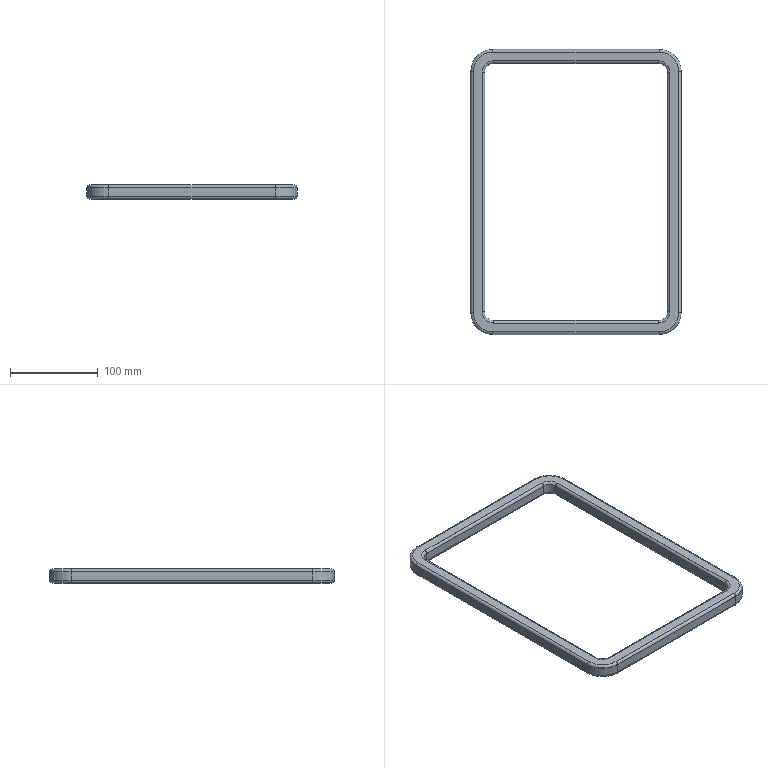Part | STEP file | Lift screen decorative outer frame 001001 | 1 solid | 100 faces | box 240 x 325 x 16 mm | volume 57771 mm3 | cylinder 48 | torus 32 | plane 20 | commonest cylinder face diameters 4 x16 6 x16 20 x4 22 x4 48 x4 50 x4